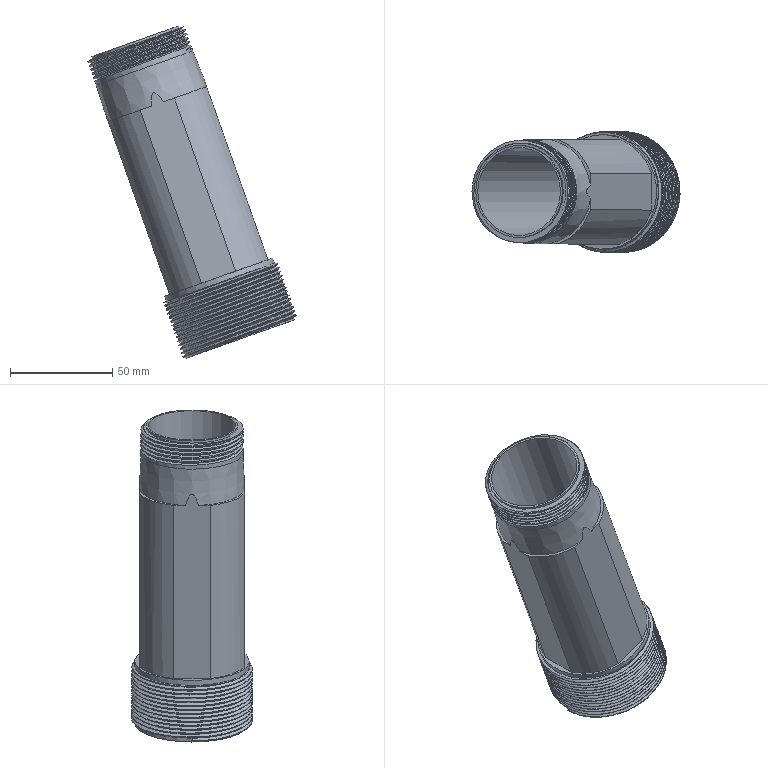Part | STEP file | SLIDE1-SCEW-AXS_id626_x_t | 1 solid | 64 faces | box 101.763 x 59.001 x 162.348 mm | volume 124425 mm3 | cylinder 27 | spline 21 | plane 15 | cone 1 | commonest cylinder face diameters 56 x15 50.086 x6 54 x4 42.96 x1 44.996 x1